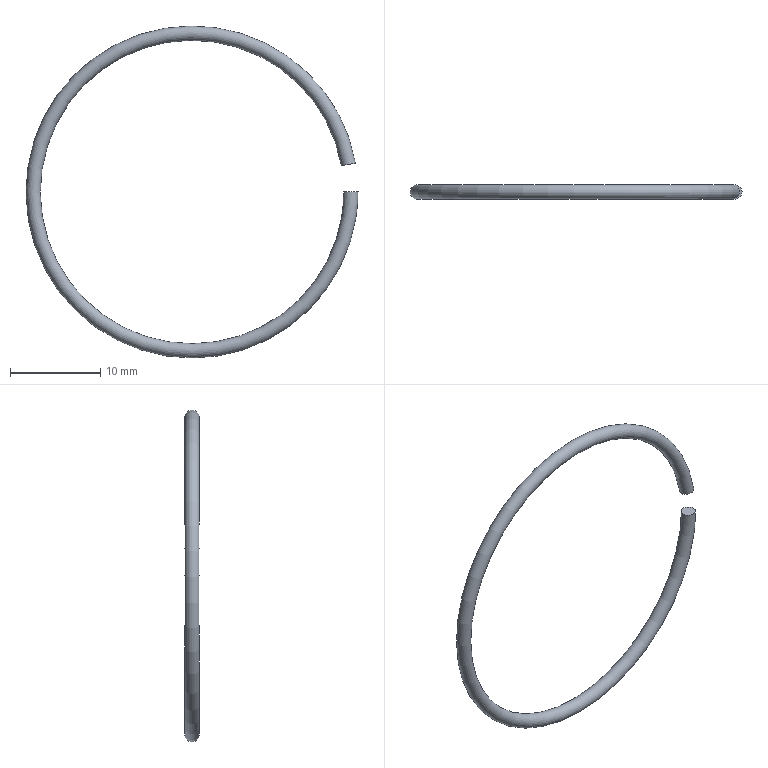Part | NX | features MG0330 trunion parts 24(stanchion group) 2 | 1 solid | 3 faces | box 36.868 x 1.588 x 36.868 mm | volume 213.289 mm3 | plane 2 | torus 1
STEP:
#1=CARTESIAN_POINT('',(18.154,281.94,3.201));
#2=VERTEX_POINT('',#1);
#3=CARTESIAN_POINT('',(17.372,281.94,3.063));
#4=DIRECTION('',(-0.1736,0.,0.9848));
#5=DIRECTION('',(0.9848,0.,0.1736));
#6=AXIS2_PLACEMENT_3D('',#3,#4,#5);
#7=CIRCLE('',#6,0.7937);
#8=EDGE_CURVE('',#2,#2,#7,.T.);
#9=ORIENTED_EDGE('',*,*,#8,.F.);
#10=EDGE_LOOP('',(#9));
#11=FACE_BOUND('',#10,.T.);
#12=CARTESIAN_POINT('',(17.372,281.94,3.063));
#13=DIRECTION('',(-0.1736,0.,0.9848));
#14=DIRECTION('',(0.9848,0.,0.1736));
#15=AXIS2_PLACEMENT_3D('',#12,#13,#14);
#16=PLANE('',#15);
#17=ADVANCED_FACE('',(#11),#16,.F.);
#18=ORIENTED_EDGE('',*,*,#8,.T.);
#19=EDGE_LOOP('',(#18));
#20=FACE_BOUND('',#19,.T.);
#21=CARTESIAN_POINT('',(18.434,281.94,0.));
#22=VERTEX_POINT('',#21);
#23=CARTESIAN_POINT('',(17.64,281.94,0.));
#24=DIRECTION('',(0.,0.,1.));
#25=DIRECTION('',(1.,0.,0.));
#26=AXIS2_PLACEMENT_3D('',#23,#24,#25);
#27=CIRCLE('',#26,0.7937);
#28=EDGE_CURVE('',#22,#22,#27,.T.);
#29=ORIENTED_EDGE('',*,*,#28,.F.);
#30=EDGE_LOOP('',(#29));
#31=FACE_BOUND('',#30,.T.);
#32=CARTESIAN_POINT('',(0.,281.94,0.));
#33=DIRECTION('',(0.,-1.,0.));
#34=DIRECTION('',(0.,0.,-1.));
#35=AXIS2_PLACEMENT_3D('',#32,#33,#34);
#36=TOROIDAL_SURFACE('',#35,17.64,0.7937);
#37=ADVANCED_FACE('',(#20,#31),#36,.T.);
#38=ORIENTED_EDGE('',*,*,#28,.T.);
#39=EDGE_LOOP('',(#38));
#40=FACE_BOUND('',#39,.T.);
#41=CARTESIAN_POINT('',(17.64,281.94,0.));
#42=DIRECTION('',(0.,0.,1.));
#43=DIRECTION('',(1.,0.,0.));
#44=AXIS2_PLACEMENT_3D('',#41,#42,#43);
#45=PLANE('',#44);
#46=ADVANCED_FACE('',(#40),#45,.T.);
#47=CLOSED_SHELL('',(#17,#37,#46));
#48=MANIFOLD_SOLID_BREP('',#47);
#49=(LENGTH_UNIT()NAMED_UNIT(*)SI_UNIT(.MILLI.,.METRE.));
#50=UNCERTAINTY_MEASURE_WITH_UNIT(LENGTH_MEASURE(0.00001),#49,'','');
#51=(NAMED_UNIT(*)PLANE_ANGLE_UNIT()SI_UNIT($,.RADIAN.));
#52=(NAMED_UNIT(*)SI_UNIT($,.STERADIAN.)SOLID_ANGLE_UNIT());
#53=(GEOMETRIC_REPRESENTATION_CONTEXT(3)GLOBAL_UNCERTAINTY_ASSIGNED_CONTEXT((#50))GLOBAL_UNIT_ASSIGNED_CONTEXT((#49,#51,#52))REPRESENTATION_CONTEXT('',''));
#54=ADVANCED_BREP_SHAPE_REPRESENTATION('',(#48),#53);